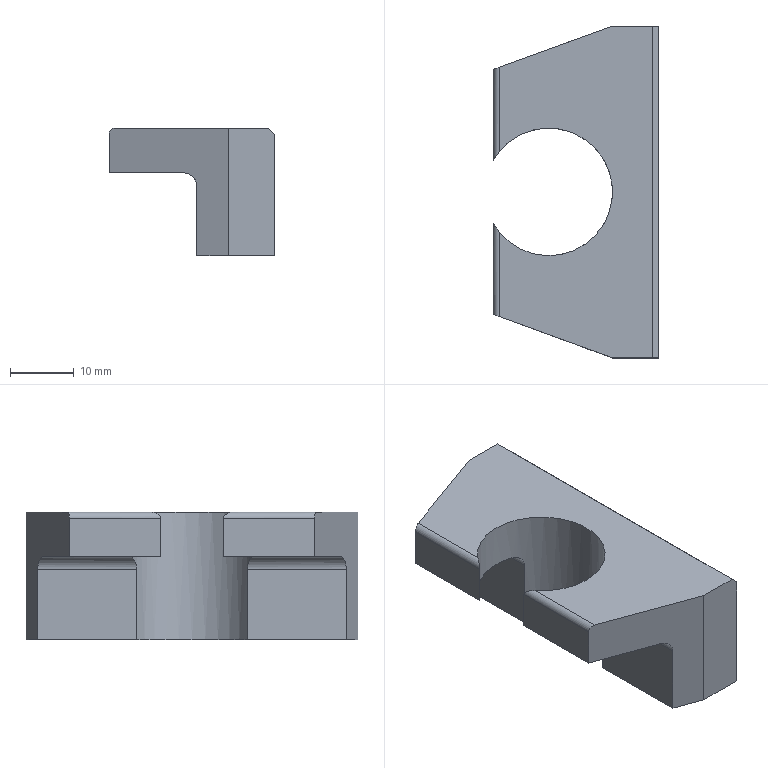Part | NX | features solid 2 | 1 solid | 19 faces | box 26 x 52 x 20 mm | volume 13805 mm3 | plane 14 | cylinder 5 | commonest cylinder face diameters 2 x2 4 x2 20 x1
STEP:
#1=CARTESIAN_POINT('',(-430.724,-194.816,182.062));
#2=VERTEX_POINT('',#1);
#3=CARTESIAN_POINT('',(-430.724,-209.119,182.062));
#4=VERTEX_POINT('',#3);
#5=CARTESIAN_POINT('',(-430.724,-188.,182.062));
#6=DIRECTION('',(0.,-1.,0.));
#7=VECTOR('',#6,1000.);
#8=LINE('',#5,#7);
#9=EDGE_CURVE('',#2,#4,#8,.T.);
#10=ORIENTED_EDGE('',*,*,#9,.F.);
#11=CARTESIAN_POINT('',(-419.,-190.549,182.062));
#12=VERTEX_POINT('',#11);
#13=CARTESIAN_POINT('',(-428.533,-194.019,182.062));
#14=DIRECTION('',(0.9397,0.342,0.));
#15=VECTOR('',#14,1000.);
#16=LINE('',#13,#15);
#17=EDGE_CURVE('',#2,#12,#16,.T.);
#18=ORIENTED_EDGE('',*,*,#17,.T.);
#19=CARTESIAN_POINT('',(-419.,-204.459,182.062));
#20=VERTEX_POINT('',#19);
#21=CARTESIAN_POINT('',(-419.,-188.,182.062));
#22=DIRECTION('',(0.,-1.,0.));
#23=VECTOR('',#22,1000.);
#24=LINE('',#21,#23);
#25=EDGE_CURVE('',#12,#20,#24,.T.);
#26=ORIENTED_EDGE('',*,*,#25,.T.);
#27=CARTESIAN_POINT('',(-421.996,-214.,182.062));
#28=DIRECTION('',(0.,0.,-1.));
#29=DIRECTION('',(-1.,0.,0.));
#30=AXIS2_PLACEMENT_3D('',#27,#28,#29);
#31=CIRCLE('',#30,10.);
#32=EDGE_CURVE('',#4,#20,#31,.T.);
#33=ORIENTED_EDGE('',*,*,#32,.F.);
#34=EDGE_LOOP('',(#10,#18,#26,#33));
#35=FACE_BOUND('',#34,.T.);
#36=CARTESIAN_POINT('',(-430.724,-188.,182.062));
#37=DIRECTION('',(0.,0.,-1.));
#38=DIRECTION('',(-1.,0.,0.));
#39=AXIS2_PLACEMENT_3D('',#36,#37,#38);
#40=PLANE('',#39);
#41=ADVANCED_FACE('',(#35),#40,.T.);
#42=CARTESIAN_POINT('',(-417.,-189.821,169.062));
#43=VERTEX_POINT('',#42);
#44=CARTESIAN_POINT('',(-417.,-189.821,180.062));
#45=VERTEX_POINT('',#44);
#46=CARTESIAN_POINT('',(-417.,-189.821,169.062));
#47=DIRECTION('',(0.,0.,1.));
#48=VECTOR('',#47,1000.);
#49=LINE('',#46,#48);
#50=EDGE_CURVE('',#43,#45,#49,.T.);
#51=ORIENTED_EDGE('',*,*,#50,.F.);
#52=CARTESIAN_POINT('',(-417.,-205.338,169.062));
#53=VERTEX_POINT('',#52);
#54=CARTESIAN_POINT('',(-417.,-188.,169.062));
#55=DIRECTION('',(0.,-1.,0.));
#56=VECTOR('',#55,1000.);
#57=LINE('',#54,#56);
#58=EDGE_CURVE('',#43,#53,#57,.T.);
#59=ORIENTED_EDGE('',*,*,#58,.T.);
#60=CARTESIAN_POINT('',(-417.,-205.338,180.062));
#61=VERTEX_POINT('',#60);
#62=CARTESIAN_POINT('',(-417.,-205.338,138.));
#63=DIRECTION('',(0.,0.,1.));
#64=VECTOR('',#63,1000.);
#65=LINE('',#62,#64);
#66=EDGE_CURVE('',#53,#61,#65,.T.);
#67=ORIENTED_EDGE('',*,*,#66,.T.);
#68=CARTESIAN_POINT('',(-417.,-188.,180.062));
#69=DIRECTION('',(0.,-1.,0.));
#70=VECTOR('',#69,1000.);
#71=LINE('',#68,#70);
#72=EDGE_CURVE('',#45,#61,#71,.T.);
#73=ORIENTED_EDGE('',*,*,#72,.F.);
#74=EDGE_LOOP('',(#51,#59,#67,#73));
#75=FACE_BOUND('',#74,.T.);
#76=CARTESIAN_POINT('',(-417.,-188.,169.062));
#77=DIRECTION('',(1.,0.,0.));
#78=DIRECTION('',(0.,0.,-1.));
#79=AXIS2_PLACEMENT_3D('',#76,#77,#78);
#80=PLANE('',#79);
#81=ADVANCED_FACE('',(#75),#80,.F.);
#82=CARTESIAN_POINT('',(-430.724,-194.816,188.062));
#83=VERTEX_POINT('',#82);
#84=CARTESIAN_POINT('',(-430.724,-194.816,182.062));
#85=DIRECTION('',(0.,0.,1.));
#86=VECTOR('',#85,1000.);
#87=LINE('',#84,#86);
#88=EDGE_CURVE('',#2,#83,#87,.T.);
#89=ORIENTED_EDGE('',*,*,#88,.F.);
#90=ORIENTED_EDGE('',*,*,#9,.T.);
#91=CARTESIAN_POINT('',(-430.724,-209.119,188.062));
#92=VERTEX_POINT('',#91);
#93=CARTESIAN_POINT('',(-430.724,-209.119,138.));
#94=DIRECTION('',(0.,0.,1.));
#95=VECTOR('',#94,1000.);
#96=LINE('',#93,#95);
#97=EDGE_CURVE('',#4,#92,#96,.T.);
#98=ORIENTED_EDGE('',*,*,#97,.T.);
#99=CARTESIAN_POINT('',(-430.724,-188.,188.062));
#100=DIRECTION('',(0.,-1.,0.));
#101=VECTOR('',#100,1000.);
#102=LINE('',#99,#101);
#103=EDGE_CURVE('',#83,#92,#102,.T.);
#104=ORIENTED_EDGE('',*,*,#103,.F.);
#105=EDGE_LOOP('',(#89,#90,#98,#104));
#106=FACE_BOUND('',#105,.T.);
#107=CARTESIAN_POINT('',(-430.724,-188.,182.062));
#108=DIRECTION('',(1.,0.,0.));
#109=DIRECTION('',(0.,0.,-1.));
#110=AXIS2_PLACEMENT_3D('',#107,#108,#109);
#111=PLANE('',#110);
#112=ADVANCED_FACE('',(#106),#111,.F.);
#113=CARTESIAN_POINT('',(-419.,-190.549,180.062));
#114=DIRECTION('',(-0.342,0.9397,0.));
#115=DIRECTION('',(-0.9397,-0.342,0.));
#116=AXIS2_PLACEMENT_3D('',#113,#114,#115);
#117=ELLIPSE('',#116,2.128,2.);
#118=EDGE_CURVE('',#45,#12,#117,.F.);
#119=ORIENTED_EDGE('',*,*,#118,.F.);
#120=ORIENTED_EDGE('',*,*,#72,.T.);
#121=CARTESIAN_POINT('',(-417.,-205.338,180.062));
#122=CARTESIAN_POINT('',(-417.,-205.338,181.166));
#123=CARTESIAN_POINT('',(-417.949,-204.79,182.062));
#124=CARTESIAN_POINT('',(-419.,-204.459,182.062));
#125=B_SPLINE_CURVE_WITH_KNOTS('',3,(#121,#122,#123,#124),.UNSPECIFIED.,.F.,.F.,(4,4),(0.,0.003261),.UNSPECIFIED.);
#126=EDGE_CURVE('',#61,#20,#125,.T.);
#127=ORIENTED_EDGE('',*,*,#126,.T.);
#128=ORIENTED_EDGE('',*,*,#25,.F.);
#129=EDGE_LOOP('',(#119,#120,#127,#128));
#130=FACE_BOUND('',#129,.T.);
#131=CARTESIAN_POINT('',(-419.,-188.,180.062));
#132=DIRECTION('',(0.,-1.,0.));
#133=DIRECTION('',(0.,0.,-1.));
#134=AXIS2_PLACEMENT_3D('',#131,#132,#133);
#135=CYLINDRICAL_SURFACE('',#134,2.);
#136=ADVANCED_FACE('',(#130),#135,.F.);
#137=ORIENTED_EDGE('',*,*,#58,.F.);
#138=CARTESIAN_POINT('',(-411.996,-188.,169.062));
#139=VERTEX_POINT('',#138);
#140=CARTESIAN_POINT('',(-416.415,-189.608,169.062));
#141=DIRECTION('',(0.9397,0.342,0.));
#142=VECTOR('',#141,1000.);
#143=LINE('',#140,#142);
#144=EDGE_CURVE('',#43,#139,#143,.T.);
#145=ORIENTED_EDGE('',*,*,#144,.T.);
#146=CARTESIAN_POINT('',(-404.724,-188.,169.062));
#147=VERTEX_POINT('',#146);
#148=CARTESIAN_POINT('',(-417.,-188.,169.062));
#149=DIRECTION('',(1.,0.,0.));
#150=VECTOR('',#149,1000.);
#151=LINE('',#148,#150);
#152=EDGE_CURVE('',#139,#147,#151,.T.);
#153=ORIENTED_EDGE('',*,*,#152,.T.);
#154=CARTESIAN_POINT('',(-404.724,-240.,169.062));
#155=VERTEX_POINT('',#154);
#156=CARTESIAN_POINT('',(-404.724,-188.,169.062));
#157=DIRECTION('',(0.,-1.,0.));
#158=VECTOR('',#157,1000.);
#159=LINE('',#156,#158);
#160=EDGE_CURVE('',#147,#155,#159,.T.);
#161=ORIENTED_EDGE('',*,*,#160,.T.);
#162=CARTESIAN_POINT('',(-411.996,-240.,169.062));
#163=VERTEX_POINT('',#162);
#164=CARTESIAN_POINT('',(-417.,-240.,169.062));
#165=DIRECTION('',(1.,0.,0.));
#166=VECTOR('',#165,1000.);
#167=LINE('',#164,#166);
#168=EDGE_CURVE('',#163,#155,#167,.T.);
#169=ORIENTED_EDGE('',*,*,#168,.F.);
#170=CARTESIAN_POINT('',(-417.,-238.179,169.062));
#171=VERTEX_POINT('',#170);
#172=CARTESIAN_POINT('',(-433.127,-232.309,169.062));
#173=DIRECTION('',(0.9397,-0.342,0.));
#174=VECTOR('',#173,1000.);
#175=LINE('',#172,#174);
#176=EDGE_CURVE('',#171,#163,#175,.T.);
#177=ORIENTED_EDGE('',*,*,#176,.F.);
#178=CARTESIAN_POINT('',(-417.,-222.662,169.062));
#179=VERTEX_POINT('',#178);
#180=CARTESIAN_POINT('',(-417.,-188.,169.062));
#181=DIRECTION('',(0.,-1.,0.));
#182=VECTOR('',#181,1000.);
#183=LINE('',#180,#182);
#184=EDGE_CURVE('',#179,#171,#183,.T.);
#185=ORIENTED_EDGE('',*,*,#184,.F.);
#186=CARTESIAN_POINT('',(-421.996,-214.,169.062));
#187=DIRECTION('',(0.,0.,-1.));
#188=DIRECTION('',(-1.,0.,0.));
#189=AXIS2_PLACEMENT_3D('',#186,#187,#188);
#190=CIRCLE('',#189,10.);
#191=EDGE_CURVE('',#53,#179,#190,.T.);
#192=ORIENTED_EDGE('',*,*,#191,.F.);
#193=EDGE_LOOP('',(#137,#145,#153,#161,#169,#177,#185,#192));
#194=FACE_BOUND('',#193,.T.);
#195=CARTESIAN_POINT('',(-417.,-188.,169.062));
#196=DIRECTION('',(0.,0.,-1.));
#197=DIRECTION('',(-1.,0.,0.));
#198=AXIS2_PLACEMENT_3D('',#195,#196,#197);
#199=PLANE('',#198);
#200=ADVANCED_FACE('',(#194),#199,.T.);
#201=CARTESIAN_POINT('',(-429.724,-194.452,189.062));
#202=VERTEX_POINT('',#201);
#203=CARTESIAN_POINT('',(-411.996,-188.,189.062));
#204=VERTEX_POINT('',#203);
#205=CARTESIAN_POINT('',(-427.65,-193.698,189.062));
#206=DIRECTION('',(0.9397,0.342,0.));
#207=VECTOR('',#206,1000.);
#208=LINE('',#205,#207);
#209=EDGE_CURVE('',#202,#204,#208,.T.);
#210=ORIENTED_EDGE('',*,*,#209,.F.);
#211=CARTESIAN_POINT('',(-429.724,-207.653,189.062));
#212=VERTEX_POINT('',#211);
#213=CARTESIAN_POINT('',(-429.724,-188.,189.062));
#214=DIRECTION('',(0.,-1.,0.));
#215=VECTOR('',#214,1000.);
#216=LINE('',#213,#215);
#217=EDGE_CURVE('',#202,#212,#216,.T.);
#218=ORIENTED_EDGE('',*,*,#217,.T.);
#219=CARTESIAN_POINT('',(-429.724,-220.347,189.062));
#220=VERTEX_POINT('',#219);
#221=CARTESIAN_POINT('',(-421.996,-214.,189.062));
#222=DIRECTION('',(0.,0.,-1.));
#223=DIRECTION('',(-1.,0.,0.));
#224=AXIS2_PLACEMENT_3D('',#221,#222,#223);
#225=CIRCLE('',#224,10.);
#226=EDGE_CURVE('',#212,#220,#225,.T.);
#227=ORIENTED_EDGE('',*,*,#226,.T.);
#228=CARTESIAN_POINT('',(-429.724,-233.548,189.062));
#229=VERTEX_POINT('',#228);
#230=CARTESIAN_POINT('',(-429.724,-188.,189.062));
#231=DIRECTION('',(0.,-1.,0.));
#232=VECTOR('',#231,1000.);
#233=LINE('',#230,#232);
#234=EDGE_CURVE('',#220,#229,#233,.T.);
#235=ORIENTED_EDGE('',*,*,#234,.T.);
#236=CARTESIAN_POINT('',(-411.996,-240.,189.062));
#237=VERTEX_POINT('',#236);
#238=CARTESIAN_POINT('',(-444.363,-228.22,189.062));
#239=DIRECTION('',(0.9397,-0.342,0.));
#240=VECTOR('',#239,1000.);
#241=LINE('',#238,#240);
#242=EDGE_CURVE('',#229,#237,#241,.T.);
#243=ORIENTED_EDGE('',*,*,#242,.T.);
#244=CARTESIAN_POINT('',(-405.724,-240.,189.062));
#245=VERTEX_POINT('',#244);
#246=CARTESIAN_POINT('',(-429.724,-240.,189.062));
#247=DIRECTION('',(1.,0.,0.));
#248=VECTOR('',#247,1000.);
#249=LINE('',#246,#248);
#250=EDGE_CURVE('',#237,#245,#249,.T.);
#251=ORIENTED_EDGE('',*,*,#250,.T.);
#252=CARTESIAN_POINT('',(-405.724,-188.,189.062));
#253=VERTEX_POINT('',#252);
#254=CARTESIAN_POINT('',(-405.724,-188.,189.062));
#255=DIRECTION('',(0.,-1.,0.));
#256=VECTOR('',#255,1000.);
#257=LINE('',#254,#256);
#258=EDGE_CURVE('',#253,#245,#257,.T.);
#259=ORIENTED_EDGE('',*,*,#258,.F.);
#260=CARTESIAN_POINT('',(-429.724,-188.,189.062));
#261=DIRECTION('',(1.,0.,0.));
#262=VECTOR('',#261,1000.);
#263=LINE('',#260,#262);
#264=EDGE_CURVE('',#204,#253,#263,.T.);
#265=ORIENTED_EDGE('',*,*,#264,.F.);
#266=EDGE_LOOP('',(#210,#218,#227,#235,#243,#251,#259,#265));
#267=FACE_BOUND('',#266,.T.);
#268=CARTESIAN_POINT('',(-429.724,-188.,189.062));
#269=DIRECTION('',(0.,0.,-1.));
#270=DIRECTION('',(-1.,0.,0.));
#271=AXIS2_PLACEMENT_3D('',#268,#269,#270);
#272=PLANE('',#271);
#273=ADVANCED_FACE('',(#267),#272,.F.);
#274=ORIENTED_EDGE('',*,*,#217,.F.);
#275=CARTESIAN_POINT('',(-429.724,-194.452,188.062));
#276=DIRECTION('',(-0.342,0.9397,0.));
#277=DIRECTION('',(-0.9397,-0.342,0.));
#278=AXIS2_PLACEMENT_3D('',#275,#276,#277);
#279=ELLIPSE('',#278,1.064,1.);
#280=EDGE_CURVE('',#202,#83,#279,.F.);
#281=ORIENTED_EDGE('',*,*,#280,.T.);
#282=ORIENTED_EDGE('',*,*,#103,.T.);
#283=CARTESIAN_POINT('',(-429.724,-207.653,189.062));
#284=CARTESIAN_POINT('',(-429.959,-207.939,189.062));
#285=CARTESIAN_POINT('',(-430.28,-208.379,188.947));
#286=CARTESIAN_POINT('',(-430.617,-208.926,188.578));
#287=CARTESIAN_POINT('',(-430.724,-209.119,188.249));
#288=CARTESIAN_POINT('',(-430.724,-209.119,188.062));
#289=B_SPLINE_CURVE_WITH_KNOTS('',3,(#283,#284,#285,#286,#287,#288),.UNSPECIFIED.,.F.,.F.,(4,1,1,4),(0.,0.001093,0.001639,0.002185),.UNSPECIFIED.);
#290=EDGE_CURVE('',#212,#92,#289,.T.);
#291=ORIENTED_EDGE('',*,*,#290,.F.);
#292=EDGE_LOOP('',(#274,#281,#282,#291));
#293=FACE_BOUND('',#292,.T.);
#294=CARTESIAN_POINT('',(-429.724,-188.,188.062));
#295=DIRECTION('',(0.,-1.,0.));
#296=DIRECTION('',(0.,0.,-1.));
#297=AXIS2_PLACEMENT_3D('',#294,#295,#296);
#298=CYLINDRICAL_SURFACE('',#297,1.);
#299=ADVANCED_FACE('',(#293),#298,.T.);
#300=CARTESIAN_POINT('',(-411.996,-188.,180.062));
#301=DIRECTION('',(0.,0.,-1.));
#302=VECTOR('',#301,1000.);
#303=LINE('',#300,#302);
#304=EDGE_CURVE('',#204,#139,#303,.T.);
#305=ORIENTED_EDGE('',*,*,#304,.F.);
#306=ORIENTED_EDGE('',*,*,#264,.T.);
#307=CARTESIAN_POINT('',(-404.724,-188.,188.062));
#308=VERTEX_POINT('',#307);
#309=CARTESIAN_POINT('',(-404.724,-188.,188.062));
#310=DIRECTION('',(-0.7071,0.,0.7071));
#311=VECTOR('',#310,1000.);
#312=LINE('',#309,#311);
#313=EDGE_CURVE('',#308,#253,#312,.T.);
#314=ORIENTED_EDGE('',*,*,#313,.F.);
#315=CARTESIAN_POINT('',(-404.724,-188.,169.062));
#316=DIRECTION('',(0.,0.,1.));
#317=VECTOR('',#316,1000.);
#318=LINE('',#315,#317);
#319=EDGE_CURVE('',#147,#308,#318,.T.);
#320=ORIENTED_EDGE('',*,*,#319,.F.);
#321=ORIENTED_EDGE('',*,*,#152,.F.);
#322=EDGE_LOOP('',(#305,#306,#314,#320,#321));
#323=FACE_BOUND('',#322,.T.);
#324=CARTESIAN_POINT('',(-419.,-188.,180.062));
#325=DIRECTION('',(0.,-1.,0.));
#326=DIRECTION('',(0.,0.,-1.));
#327=AXIS2_PLACEMENT_3D('',#324,#325,#326);
#328=PLANE('',#327);
#329=ADVANCED_FACE('',(#323),#328,.F.);
#330=CARTESIAN_POINT('',(-417.,-222.662,180.062));
#331=VERTEX_POINT('',#330);
#332=CARTESIAN_POINT('',(-417.,-238.179,180.062));
#333=VERTEX_POINT('',#332);
#334=CARTESIAN_POINT('',(-417.,-188.,180.062));
#335=DIRECTION('',(0.,-1.,0.));
#336=VECTOR('',#335,1000.);
#337=LINE('',#334,#336);
#338=EDGE_CURVE('',#331,#333,#337,.T.);
#339=ORIENTED_EDGE('',*,*,#338,.T.);
#340=CARTESIAN_POINT('',(-419.,-237.451,182.062));
#341=VERTEX_POINT('',#340);
#342=CARTESIAN_POINT('',(-419.,-237.451,180.062));
#343=DIRECTION('',(0.342,0.9397,0.));
#344=DIRECTION('',(0.9397,-0.342,0.));
#345=AXIS2_PLACEMENT_3D('',#342,#343,#344);
#346=ELLIPSE('',#345,2.128,2.);
#347=EDGE_CURVE('',#333,#341,#346,.F.);
#348=ORIENTED_EDGE('',*,*,#347,.T.);
#349=CARTESIAN_POINT('',(-419.,-223.541,182.062));
#350=VERTEX_POINT('',#349);
#351=CARTESIAN_POINT('',(-419.,-188.,182.062));
#352=DIRECTION('',(0.,-1.,0.));
#353=VECTOR('',#352,1000.);
#354=LINE('',#351,#353);
#355=EDGE_CURVE('',#350,#341,#354,.T.);
#356=ORIENTED_EDGE('',*,*,#355,.F.);
#357=CARTESIAN_POINT('',(-419.,-223.541,182.062));
#358=CARTESIAN_POINT('',(-417.947,-223.21,182.062));
#359=CARTESIAN_POINT('',(-417.,-222.662,181.169));
#360=CARTESIAN_POINT('',(-417.,-222.662,180.062));
#361=B_SPLINE_CURVE_WITH_KNOTS('',3,(#357,#358,#359,#360),.UNSPECIFIED.,.F.,.F.,(4,4),(0.,0.003262),.UNSPECIFIED.);
#362=EDGE_CURVE('',#350,#331,#361,.T.);
#363=ORIENTED_EDGE('',*,*,#362,.T.);
#364=EDGE_LOOP('',(#339,#348,#356,#363));
#365=FACE_BOUND('',#364,.T.);
#366=CARTESIAN_POINT('',(-419.,-188.,180.062));
#367=DIRECTION('',(0.,-1.,0.));
#368=DIRECTION('',(0.,0.,-1.));
#369=AXIS2_PLACEMENT_3D('',#366,#367,#368);
#370=CYLINDRICAL_SURFACE('',#369,2.);
#371=ADVANCED_FACE('',(#365),#370,.F.);
#372=CARTESIAN_POINT('',(-430.724,-233.184,188.062));
#373=VERTEX_POINT('',#372);
#374=CARTESIAN_POINT('',(-429.724,-233.548,188.062));
#375=DIRECTION('',(0.342,0.9397,0.));
#376=DIRECTION('',(0.9397,-0.342,0.));
#377=AXIS2_PLACEMENT_3D('',#374,#375,#376);
#378=ELLIPSE('',#377,1.064,1.);
#379=EDGE_CURVE('',#229,#373,#378,.F.);
#380=ORIENTED_EDGE('',*,*,#379,.F.);
#381=ORIENTED_EDGE('',*,*,#234,.F.);
#382=CARTESIAN_POINT('',(-430.724,-218.881,188.062));
#383=VERTEX_POINT('',#382);
#384=CARTESIAN_POINT('',(-430.724,-218.881,188.062));
#385=CARTESIAN_POINT('',(-430.724,-218.881,188.25));
#386=CARTESIAN_POINT('',(-430.617,-219.074,188.578));
#387=CARTESIAN_POINT('',(-430.28,-219.619,188.947));
#388=CARTESIAN_POINT('',(-429.958,-220.062,189.062));
#389=CARTESIAN_POINT('',(-429.724,-220.347,189.062));
#390=B_SPLINE_CURVE_WITH_KNOTS('',3,(#384,#385,#386,#387,#388,#389),.UNSPECIFIED.,.F.,.F.,(4,1,1,4),(0.,0.0005526,0.001105,0.00221),.UNSPECIFIED.);
#391=EDGE_CURVE('',#383,#220,#390,.T.);
#392=ORIENTED_EDGE('',*,*,#391,.F.);
#393=CARTESIAN_POINT('',(-430.724,-188.,188.062));
#394=DIRECTION('',(0.,-1.,0.));
#395=VECTOR('',#394,1000.);
#396=LINE('',#393,#395);
#397=EDGE_CURVE('',#383,#373,#396,.T.);
#398=ORIENTED_EDGE('',*,*,#397,.T.);
#399=EDGE_LOOP('',(#380,#381,#392,#398));
#400=FACE_BOUND('',#399,.T.);
#401=CARTESIAN_POINT('',(-429.724,-188.,188.062));
#402=DIRECTION('',(0.,-1.,0.));
#403=DIRECTION('',(0.,0.,-1.));
#404=AXIS2_PLACEMENT_3D('',#401,#402,#403);
#405=CYLINDRICAL_SURFACE('',#404,1.);
#406=ADVANCED_FACE('',(#400),#405,.T.);
#407=CARTESIAN_POINT('',(-430.724,-233.184,182.062));
#408=VERTEX_POINT('',#407);
#409=CARTESIAN_POINT('',(-445.246,-227.898,182.062));
#410=DIRECTION('',(0.9397,-0.342,0.));
#411=VECTOR('',#410,1000.);
#412=LINE('',#409,#411);
#413=EDGE_CURVE('',#408,#341,#412,.T.);
#414=ORIENTED_EDGE('',*,*,#413,.F.);
#415=CARTESIAN_POINT('',(-430.724,-218.881,182.062));
#416=VERTEX_POINT('',#415);
#417=CARTESIAN_POINT('',(-430.724,-188.,182.062));
#418=DIRECTION('',(0.,-1.,0.));
#419=VECTOR('',#418,1000.);
#420=LINE('',#417,#419);
#421=EDGE_CURVE('',#416,#408,#420,.T.);
#422=ORIENTED_EDGE('',*,*,#421,.F.);
#423=CARTESIAN_POINT('',(-421.996,-214.,182.062));
#424=DIRECTION('',(0.,0.,-1.));
#425=DIRECTION('',(-1.,0.,0.));
#426=AXIS2_PLACEMENT_3D('',#423,#424,#425);
#427=CIRCLE('',#426,10.);
#428=EDGE_CURVE('',#350,#416,#427,.T.);
#429=ORIENTED_EDGE('',*,*,#428,.F.);
#430=ORIENTED_EDGE('',*,*,#355,.T.);
#431=EDGE_LOOP('',(#414,#422,#429,#430));
#432=FACE_BOUND('',#431,.T.);
#433=CARTESIAN_POINT('',(-430.724,-188.,182.062));
#434=DIRECTION('',(0.,0.,-1.));
#435=DIRECTION('',(-1.,0.,0.));
#436=AXIS2_PLACEMENT_3D('',#433,#434,#435);
#437=PLANE('',#436);
#438=ADVANCED_FACE('',(#432),#437,.T.);
#439=ORIENTED_EDGE('',*,*,#184,.T.);
#440=CARTESIAN_POINT('',(-417.,-238.179,169.062));
#441=DIRECTION('',(0.,0.,1.));
#442=VECTOR('',#441,1000.);
#443=LINE('',#440,#442);
#444=EDGE_CURVE('',#171,#333,#443,.T.);
#445=ORIENTED_EDGE('',*,*,#444,.T.);
#446=ORIENTED_EDGE('',*,*,#338,.F.);
#447=CARTESIAN_POINT('',(-417.,-222.662,138.));
#448=DIRECTION('',(0.,0.,1.));
#449=VECTOR('',#448,1000.);
#450=LINE('',#447,#449);
#451=EDGE_CURVE('',#331,#179,#450,.F.);
#452=ORIENTED_EDGE('',*,*,#451,.T.);
#453=EDGE_LOOP('',(#439,#445,#446,#452));
#454=FACE_BOUND('',#453,.T.);
#455=CARTESIAN_POINT('',(-417.,-188.,169.062));
#456=DIRECTION('',(1.,0.,0.));
#457=DIRECTION('',(0.,0.,-1.));
#458=AXIS2_PLACEMENT_3D('',#455,#456,#457);
#459=PLANE('',#458);
#460=ADVANCED_FACE('',(#454),#459,.F.);
#461=CARTESIAN_POINT('',(-404.724,-240.,188.062));
#462=VERTEX_POINT('',#461);
#463=CARTESIAN_POINT('',(-404.724,-240.,169.062));
#464=DIRECTION('',(0.,0.,1.));
#465=VECTOR('',#464,1000.);
#466=LINE('',#463,#465);
#467=EDGE_CURVE('',#155,#462,#466,.T.);
#468=ORIENTED_EDGE('',*,*,#467,.F.);
#469=ORIENTED_EDGE('',*,*,#160,.F.);
#470=ORIENTED_EDGE('',*,*,#319,.T.);
#471=CARTESIAN_POINT('',(-404.724,-188.,188.062));
#472=DIRECTION('',(0.,-1.,0.));
#473=VECTOR('',#472,1000.);
#474=LINE('',#471,#473);
#475=EDGE_CURVE('',#308,#462,#474,.T.);
#476=ORIENTED_EDGE('',*,*,#475,.T.);
#477=EDGE_LOOP('',(#468,#469,#470,#476));
#478=FACE_BOUND('',#477,.T.);
#479=CARTESIAN_POINT('',(-404.724,-188.,169.062));
#480=DIRECTION('',(1.,0.,0.));
#481=DIRECTION('',(0.,0.,-1.));
#482=AXIS2_PLACEMENT_3D('',#479,#480,#481);
#483=PLANE('',#482);
#484=ADVANCED_FACE('',(#478),#483,.T.);
#485=CARTESIAN_POINT('',(-404.724,-240.,188.062));
#486=DIRECTION('',(-0.7071,0.,0.7071));
#487=VECTOR('',#486,1000.);
#488=LINE('',#485,#487);
#489=EDGE_CURVE('',#462,#245,#488,.T.);
#490=ORIENTED_EDGE('',*,*,#489,.F.);
#491=ORIENTED_EDGE('',*,*,#475,.F.);
#492=ORIENTED_EDGE('',*,*,#313,.T.);
#493=ORIENTED_EDGE('',*,*,#258,.T.);
#494=EDGE_LOOP('',(#490,#491,#492,#493));
#495=FACE_BOUND('',#494,.T.);
#496=CARTESIAN_POINT('',(-404.724,-188.,188.062));
#497=DIRECTION('',(0.7071,0.,0.7071));
#498=DIRECTION('',(0.7071,0.,-0.7071));
#499=AXIS2_PLACEMENT_3D('',#496,#497,#498);
#500=PLANE('',#499);
#501=ADVANCED_FACE('',(#495),#500,.T.);
#502=ORIENTED_EDGE('',*,*,#421,.T.);
#503=CARTESIAN_POINT('',(-430.724,-233.184,182.062));
#504=DIRECTION('',(0.,0.,1.));
#505=VECTOR('',#504,1000.);
#506=LINE('',#503,#505);
#507=EDGE_CURVE('',#408,#373,#506,.T.);
#508=ORIENTED_EDGE('',*,*,#507,.T.);
#509=ORIENTED_EDGE('',*,*,#397,.F.);
#510=CARTESIAN_POINT('',(-430.724,-218.881,138.));
#511=DIRECTION('',(0.,0.,1.));
#512=VECTOR('',#511,1000.);
#513=LINE('',#510,#512);
#514=EDGE_CURVE('',#383,#416,#513,.F.);
#515=ORIENTED_EDGE('',*,*,#514,.T.);
#516=EDGE_LOOP('',(#502,#508,#509,#515));
#517=FACE_BOUND('',#516,.T.);
#518=CARTESIAN_POINT('',(-430.724,-188.,182.062));
#519=DIRECTION('',(1.,0.,0.));
#520=DIRECTION('',(0.,0.,-1.));
#521=AXIS2_PLACEMENT_3D('',#518,#519,#520);
#522=PLANE('',#521);
#523=ADVANCED_FACE('',(#517),#522,.F.);
#524=CARTESIAN_POINT('',(-411.996,-240.,180.062));
#525=DIRECTION('',(0.,0.,1.));
#526=VECTOR('',#525,1000.);
#527=LINE('',#524,#526);
#528=EDGE_CURVE('',#163,#237,#527,.T.);
#529=ORIENTED_EDGE('',*,*,#528,.F.);
#530=ORIENTED_EDGE('',*,*,#168,.T.);
#531=ORIENTED_EDGE('',*,*,#467,.T.);
#532=ORIENTED_EDGE('',*,*,#489,.T.);
#533=ORIENTED_EDGE('',*,*,#250,.F.);
#534=EDGE_LOOP('',(#529,#530,#531,#532,#533));
#535=FACE_BOUND('',#534,.T.);
#536=CARTESIAN_POINT('',(-419.,-240.,180.062));
#537=DIRECTION('',(0.,-1.,0.));
#538=DIRECTION('',(0.,0.,-1.));
#539=AXIS2_PLACEMENT_3D('',#536,#537,#538);
#540=PLANE('',#539);
#541=ADVANCED_FACE('',(#535),#540,.T.);
#542=ORIENTED_EDGE('',*,*,#66,.F.);
#543=ORIENTED_EDGE('',*,*,#191,.T.);
#544=ORIENTED_EDGE('',*,*,#451,.F.);
#545=ORIENTED_EDGE('',*,*,#362,.F.);
#546=ORIENTED_EDGE('',*,*,#428,.T.);
#547=ORIENTED_EDGE('',*,*,#514,.F.);
#548=ORIENTED_EDGE('',*,*,#391,.T.);
#549=ORIENTED_EDGE('',*,*,#226,.F.);
#550=ORIENTED_EDGE('',*,*,#290,.T.);
#551=ORIENTED_EDGE('',*,*,#97,.F.);
#552=ORIENTED_EDGE('',*,*,#32,.T.);
#553=ORIENTED_EDGE('',*,*,#126,.F.);
#554=EDGE_LOOP('',(#542,#543,#544,#545,#546,#547,#548,#549,#550,#551,#552,#553));
#555=FACE_BOUND('',#554,.T.);
#556=CARTESIAN_POINT('',(-421.996,-214.,138.));
#557=DIRECTION('',(0.,0.,1.));
#558=DIRECTION('',(1.,0.,0.));
#559=AXIS2_PLACEMENT_3D('',#556,#557,#558);
#560=CYLINDRICAL_SURFACE('',#559,10.);
#561=ADVANCED_FACE('',(#555),#560,.F.);
#562=ORIENTED_EDGE('',*,*,#507,.F.);
#563=ORIENTED_EDGE('',*,*,#413,.T.);
#564=ORIENTED_EDGE('',*,*,#347,.F.);
#565=ORIENTED_EDGE('',*,*,#444,.F.);
#566=ORIENTED_EDGE('',*,*,#176,.T.);
#567=ORIENTED_EDGE('',*,*,#528,.T.);
#568=ORIENTED_EDGE('',*,*,#242,.F.);
#569=ORIENTED_EDGE('',*,*,#379,.T.);
#570=EDGE_LOOP('',(#562,#563,#564,#565,#566,#567,#568,#569));
#571=FACE_BOUND('',#570,.T.);
#572=CARTESIAN_POINT('',(-436.996,-230.901,189.998));
#573=DIRECTION('',(0.342,0.9397,0.));
#574=DIRECTION('',(-0.9397,0.342,0.));
#575=AXIS2_PLACEMENT_3D('',#572,#573,#574);
#576=PLANE('',#575);
#577=ADVANCED_FACE('',(#571),#576,.F.);
#578=ORIENTED_EDGE('',*,*,#17,.F.);
#579=ORIENTED_EDGE('',*,*,#88,.T.);
#580=ORIENTED_EDGE('',*,*,#280,.F.);
#581=ORIENTED_EDGE('',*,*,#209,.T.);
#582=ORIENTED_EDGE('',*,*,#304,.T.);
#583=ORIENTED_EDGE('',*,*,#144,.F.);
#584=ORIENTED_EDGE('',*,*,#50,.T.);
#585=ORIENTED_EDGE('',*,*,#118,.T.);
#586=EDGE_LOOP('',(#578,#579,#580,#581,#582,#583,#584,#585));
#587=FACE_BOUND('',#586,.T.);
#588=CARTESIAN_POINT('',(-436.996,-197.099,210.));
#589=DIRECTION('',(-0.342,0.9397,0.));
#590=DIRECTION('',(-0.9397,-0.342,0.));
#591=AXIS2_PLACEMENT_3D('',#588,#589,#590);
#592=PLANE('',#591);
#593=ADVANCED_FACE('',(#587),#592,.T.);
#594=CLOSED_SHELL('',(#41,#81,#112,#136,#200,#273,#299,#329,#371,#406,#438,#460,#484,#501,#523,#541,#561,#577,#593));
#595=MANIFOLD_SOLID_BREP('',#594);
#596=(LENGTH_UNIT()NAMED_UNIT(*)SI_UNIT(.MILLI.,.METRE.));
#597=UNCERTAINTY_MEASURE_WITH_UNIT(LENGTH_MEASURE(0.0508),#596,'','');
#598=(NAMED_UNIT(*)PLANE_ANGLE_UNIT()SI_UNIT($,.RADIAN.));
#599=(NAMED_UNIT(*)SI_UNIT($,.STERADIAN.)SOLID_ANGLE_UNIT());
#600=(GEOMETRIC_REPRESENTATION_CONTEXT(3)GLOBAL_UNCERTAINTY_ASSIGNED_CONTEXT((#597))GLOBAL_UNIT_ASSIGNED_CONTEXT((#596,#598,#599))REPRESENTATION_CONTEXT('',''));
#601=ADVANCED_BREP_SHAPE_REPRESENTATION('',(#595),#600);